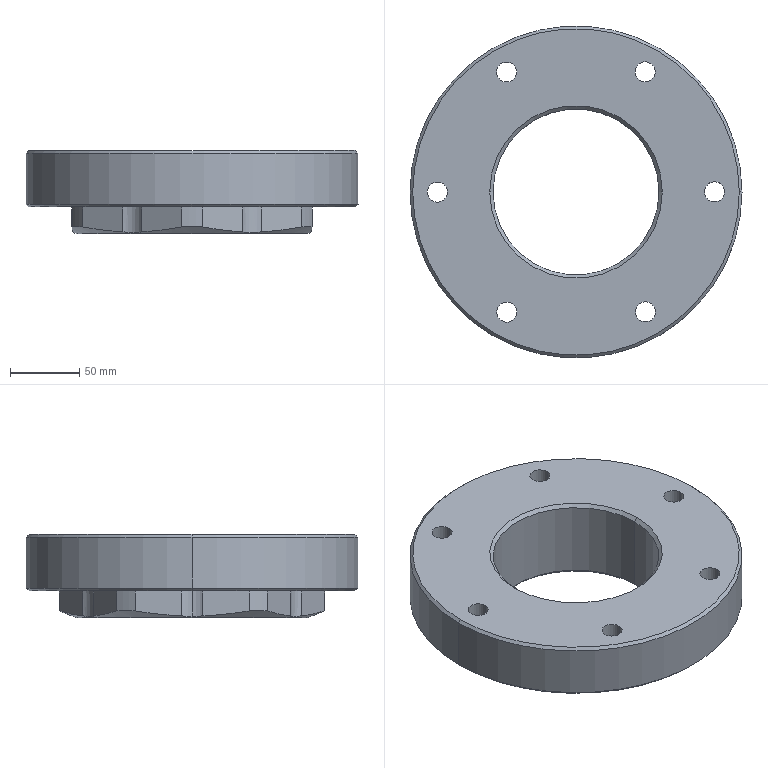Part | SolidWorks | features ICE 3, BaseBody 1, Chamfer 1, Scale 1 | 1 solid | 72 faces | box 240 x 240 x 60 mm | volume 1562798 mm3 | cylinder 41 | plane 21 | cone 10 | commonest cylinder face diameters 14.5 x12 26 x12 31.2 x7 192 x6 120 x2 240 x2